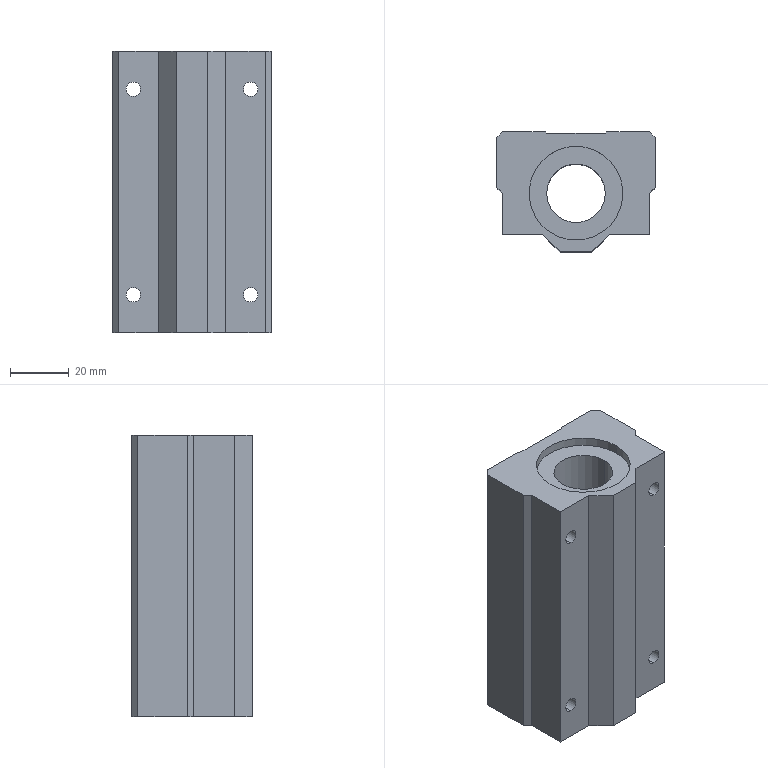Part | SolidWorks | features BaseBody 1 | 1 solid | 44 faces | box 54 x 41 x 96 mm | volume 148221 mm3 | plane 22 | cylinder 14 | cone 8 | commonest cylinder face diameters 4.917 x8 32 x4 20 x2
STEP:
#1=CARTESIAN_POINT('',(-10.,0.,-93.));
#2=VERTEX_POINT('',#1);
#3=CARTESIAN_POINT('',(10.,0.,-93.));
#4=VERTEX_POINT('',#3);
#5=CARTESIAN_POINT('',(0.,0.,-93.));
#6=DIRECTION('',(0.,0.,1.));
#7=DIRECTION('',(1.,0.,0.));
#8=AXIS2_PLACEMENT_3D('',#5,#6,#7);
#9=CIRCLE('',#8,10.);
#10=EDGE_CURVE('',#2,#4,#9,.T.);
#11=ORIENTED_EDGE('',*,*,#10,.F.);
#12=CARTESIAN_POINT('',(-10.,0.,-3.));
#13=VERTEX_POINT('',#12);
#14=CARTESIAN_POINT('',(-10.,0.,-96.));
#15=DIRECTION('',(0.,0.,1.));
#16=VECTOR('',#15,1000.);
#17=LINE('',#14,#16);
#18=EDGE_CURVE('',#2,#13,#17,.T.);
#19=ORIENTED_EDGE('',*,*,#18,.T.);
#20=CARTESIAN_POINT('',(10.,0.,-3.));
#21=VERTEX_POINT('',#20);
#22=CARTESIAN_POINT('',(0.,0.,-3.));
#23=DIRECTION('',(0.,0.,-1.));
#24=DIRECTION('',(1.,0.,0.));
#25=AXIS2_PLACEMENT_3D('',#22,#23,#24);
#26=CIRCLE('',#25,10.);
#27=EDGE_CURVE('',#21,#13,#26,.T.);
#28=ORIENTED_EDGE('',*,*,#27,.F.);
#29=CARTESIAN_POINT('',(10.,0.,-96.));
#30=DIRECTION('',(0.,0.,1.));
#31=VECTOR('',#30,1000.);
#32=LINE('',#29,#31);
#33=EDGE_CURVE('',#4,#21,#32,.T.);
#34=ORIENTED_EDGE('',*,*,#33,.F.);
#35=EDGE_LOOP('',(#11,#19,#28,#34));
#36=FACE_OUTER_BOUND('',#35,.T.);
#37=CARTESIAN_POINT('',(0.,0.,-96.));
#38=DIRECTION('',(0.,0.,1.));
#39=DIRECTION('',(1.,0.,0.));
#40=AXIS2_PLACEMENT_3D('',#37,#38,#39);
#41=CYLINDRICAL_SURFACE('',#40,10.);
#42=ADVANCED_FACE('',(#36),#41,.F.);
#43=CARTESIAN_POINT('',(-16.,0.,-3.));
#44=VERTEX_POINT('',#43);
#45=CARTESIAN_POINT('',(16.,0.,-3.));
#46=VERTEX_POINT('',#45);
#47=CARTESIAN_POINT('',(0.,0.,-3.));
#48=DIRECTION('',(0.,0.,1.));
#49=DIRECTION('',(1.,0.,0.));
#50=AXIS2_PLACEMENT_3D('',#47,#48,#49);
#51=CIRCLE('',#50,16.);
#52=EDGE_CURVE('',#44,#46,#51,.T.);
#53=ORIENTED_EDGE('',*,*,#52,.F.);
#54=CARTESIAN_POINT('',(-16.,0.,0.));
#55=VERTEX_POINT('',#54);
#56=CARTESIAN_POINT('',(-16.,0.,-96.));
#57=DIRECTION('',(0.,0.,1.));
#58=VECTOR('',#57,1000.);
#59=LINE('',#56,#58);
#60=EDGE_CURVE('',#44,#55,#59,.T.);
#61=ORIENTED_EDGE('',*,*,#60,.T.);
#62=CARTESIAN_POINT('',(16.,0.,0.));
#63=VERTEX_POINT('',#62);
#64=CARTESIAN_POINT('',(0.,0.,0.));
#65=DIRECTION('',(0.,0.,-1.));
#66=DIRECTION('',(1.,0.,0.));
#67=AXIS2_PLACEMENT_3D('',#64,#65,#66);
#68=CIRCLE('',#67,16.);
#69=EDGE_CURVE('',#63,#55,#68,.T.);
#70=ORIENTED_EDGE('',*,*,#69,.F.);
#71=CARTESIAN_POINT('',(16.,0.,-96.));
#72=DIRECTION('',(0.,0.,1.));
#73=VECTOR('',#72,1000.);
#74=LINE('',#71,#73);
#75=EDGE_CURVE('',#46,#63,#74,.T.);
#76=ORIENTED_EDGE('',*,*,#75,.F.);
#77=EDGE_LOOP('',(#53,#61,#70,#76));
#78=FACE_OUTER_BOUND('',#77,.T.);
#79=CARTESIAN_POINT('',(0.,0.,-96.));
#80=DIRECTION('',(0.,0.,1.));
#81=DIRECTION('',(1.,0.,0.));
#82=AXIS2_PLACEMENT_3D('',#79,#80,#81);
#83=CYLINDRICAL_SURFACE('',#82,16.);
#84=ADVANCED_FACE('',(#78),#83,.F.);
#85=CARTESIAN_POINT('',(-16.,0.,-96.));
#86=VERTEX_POINT('',#85);
#87=CARTESIAN_POINT('',(16.,0.,-96.));
#88=VERTEX_POINT('',#87);
#89=CARTESIAN_POINT('',(0.,0.,-96.));
#90=DIRECTION('',(0.,0.,1.));
#91=DIRECTION('',(1.,0.,0.));
#92=AXIS2_PLACEMENT_3D('',#89,#90,#91);
#93=CIRCLE('',#92,16.);
#94=EDGE_CURVE('',#86,#88,#93,.T.);
#95=ORIENTED_EDGE('',*,*,#94,.F.);
#96=CARTESIAN_POINT('',(-16.,0.,-93.));
#97=VERTEX_POINT('',#96);
#98=CARTESIAN_POINT('',(-16.,0.,-96.));
#99=DIRECTION('',(0.,0.,1.));
#100=VECTOR('',#99,1000.);
#101=LINE('',#98,#100);
#102=EDGE_CURVE('',#86,#97,#101,.T.);
#103=ORIENTED_EDGE('',*,*,#102,.T.);
#104=CARTESIAN_POINT('',(16.,0.,-93.));
#105=VERTEX_POINT('',#104);
#106=CARTESIAN_POINT('',(0.,0.,-93.));
#107=DIRECTION('',(0.,0.,-1.));
#108=DIRECTION('',(1.,0.,0.));
#109=AXIS2_PLACEMENT_3D('',#106,#107,#108);
#110=CIRCLE('',#109,16.);
#111=EDGE_CURVE('',#105,#97,#110,.T.);
#112=ORIENTED_EDGE('',*,*,#111,.F.);
#113=CARTESIAN_POINT('',(16.,0.,-96.));
#114=DIRECTION('',(0.,0.,1.));
#115=VECTOR('',#114,1000.);
#116=LINE('',#113,#115);
#117=EDGE_CURVE('',#88,#105,#116,.T.);
#118=ORIENTED_EDGE('',*,*,#117,.F.);
#119=EDGE_LOOP('',(#95,#103,#112,#118));
#120=FACE_OUTER_BOUND('',#119,.T.);
#121=CARTESIAN_POINT('',(0.,0.,-96.));
#122=DIRECTION('',(0.,0.,1.));
#123=DIRECTION('',(1.,0.,0.));
#124=AXIS2_PLACEMENT_3D('',#121,#122,#123);
#125=CYLINDRICAL_SURFACE('',#124,16.);
#126=ADVANCED_FACE('',(#120),#125,.F.);
#127=CARTESIAN_POINT('',(-20.,20.459,-85.459));
#128=VERTEX_POINT('',#127);
#129=CARTESIAN_POINT('',(-20.,20.459,-80.541));
#130=VERTEX_POINT('',#129);
#131=CARTESIAN_POINT('',(-20.,20.459,-83.));
#132=DIRECTION('',(0.,1.,0.));
#133=DIRECTION('',(0.,0.,1.));
#134=AXIS2_PLACEMENT_3D('',#131,#132,#133);
#135=CIRCLE('',#134,2.459);
#136=EDGE_CURVE('',#128,#130,#135,.T.);
#137=ORIENTED_EDGE('',*,*,#136,.F.);
#138=CARTESIAN_POINT('',(-20.,21.,-86.));
#139=VERTEX_POINT('',#138);
#140=CARTESIAN_POINT('',(-20.,21.,-86.));
#141=DIRECTION('',(0.,0.7071,-0.7071));
#142=VECTOR('',#141,1000.);
#143=LINE('',#140,#142);
#144=EDGE_CURVE('',#128,#139,#143,.T.);
#145=ORIENTED_EDGE('',*,*,#144,.T.);
#146=CARTESIAN_POINT('',(-20.,21.,-80.));
#147=VERTEX_POINT('',#146);
#148=CARTESIAN_POINT('',(-20.,21.,-83.));
#149=DIRECTION('',(0.,-1.,0.));
#150=DIRECTION('',(0.,0.,1.));
#151=AXIS2_PLACEMENT_3D('',#148,#149,#150);
#152=CIRCLE('',#151,3.);
#153=EDGE_CURVE('',#147,#139,#152,.T.);
#154=ORIENTED_EDGE('',*,*,#153,.F.);
#155=CARTESIAN_POINT('',(-20.,21.,-80.));
#156=DIRECTION('',(0.,0.7071,0.7071));
#157=VECTOR('',#156,1000.);
#158=LINE('',#155,#157);
#159=EDGE_CURVE('',#130,#147,#158,.T.);
#160=ORIENTED_EDGE('',*,*,#159,.F.);
#161=EDGE_LOOP('',(#137,#145,#154,#160));
#162=FACE_OUTER_BOUND('',#161,.T.);
#163=CARTESIAN_POINT('',(-20.,21.,-83.));
#164=DIRECTION('',(0.,1.,0.));
#165=DIRECTION('',(0.,0.,1.));
#166=AXIS2_PLACEMENT_3D('',#163,#164,#165);
#167=CONICAL_SURFACE('',#166,3.,0.7854);
#168=ADVANCED_FACE('',(#162),#167,.F.);
#169=CARTESIAN_POINT('',(-20.,20.459,-15.459));
#170=VERTEX_POINT('',#169);
#171=CARTESIAN_POINT('',(-20.,20.459,-10.541));
#172=VERTEX_POINT('',#171);
#173=CARTESIAN_POINT('',(-20.,20.459,-13.));
#174=DIRECTION('',(0.,1.,0.));
#175=DIRECTION('',(0.,0.,1.));
#176=AXIS2_PLACEMENT_3D('',#173,#174,#175);
#177=CIRCLE('',#176,2.459);
#178=EDGE_CURVE('',#170,#172,#177,.T.);
#179=ORIENTED_EDGE('',*,*,#178,.F.);
#180=CARTESIAN_POINT('',(-20.,21.,-16.));
#181=VERTEX_POINT('',#180);
#182=CARTESIAN_POINT('',(-20.,21.,-16.));
#183=DIRECTION('',(0.,0.7071,-0.7071));
#184=VECTOR('',#183,1000.);
#185=LINE('',#182,#184);
#186=EDGE_CURVE('',#170,#181,#185,.T.);
#187=ORIENTED_EDGE('',*,*,#186,.T.);
#188=CARTESIAN_POINT('',(-20.,21.,-10.));
#189=VERTEX_POINT('',#188);
#190=CARTESIAN_POINT('',(-20.,21.,-13.));
#191=DIRECTION('',(0.,-1.,0.));
#192=DIRECTION('',(0.,0.,1.));
#193=AXIS2_PLACEMENT_3D('',#190,#191,#192);
#194=CIRCLE('',#193,3.);
#195=EDGE_CURVE('',#189,#181,#194,.T.);
#196=ORIENTED_EDGE('',*,*,#195,.F.);
#197=CARTESIAN_POINT('',(-20.,21.,-10.));
#198=DIRECTION('',(0.,0.7071,0.7071));
#199=VECTOR('',#198,1000.);
#200=LINE('',#197,#199);
#201=EDGE_CURVE('',#172,#189,#200,.T.);
#202=ORIENTED_EDGE('',*,*,#201,.F.);
#203=EDGE_LOOP('',(#179,#187,#196,#202));
#204=FACE_OUTER_BOUND('',#203,.T.);
#205=CARTESIAN_POINT('',(-20.,21.,-13.));
#206=DIRECTION('',(0.,1.,0.));
#207=DIRECTION('',(0.,0.,1.));
#208=AXIS2_PLACEMENT_3D('',#205,#206,#207);
#209=CONICAL_SURFACE('',#208,3.,0.7854);
#210=ADVANCED_FACE('',(#204),#209,.F.);
#211=CARTESIAN_POINT('',(20.,20.458,-85.459));
#212=VERTEX_POINT('',#211);
#213=CARTESIAN_POINT('',(20.,20.458,-80.541));
#214=VERTEX_POINT('',#213);
#215=CARTESIAN_POINT('',(20.,20.458,-83.));
#216=DIRECTION('',(0.,1.,0.));
#217=DIRECTION('',(0.,0.,1.));
#218=AXIS2_PLACEMENT_3D('',#215,#216,#217);
#219=CIRCLE('',#218,2.459);
#220=EDGE_CURVE('',#212,#214,#219,.T.);
#221=ORIENTED_EDGE('',*,*,#220,.F.);
#222=CARTESIAN_POINT('',(20.,21.,-86.));
#223=VERTEX_POINT('',#222);
#224=CARTESIAN_POINT('',(20.,21.,-86.));
#225=DIRECTION('',(0.,0.7071,-0.7071));
#226=VECTOR('',#225,1000.);
#227=LINE('',#224,#226);
#228=EDGE_CURVE('',#212,#223,#227,.T.);
#229=ORIENTED_EDGE('',*,*,#228,.T.);
#230=CARTESIAN_POINT('',(20.,21.,-80.));
#231=VERTEX_POINT('',#230);
#232=CARTESIAN_POINT('',(20.,21.,-83.));
#233=DIRECTION('',(0.,-1.,0.));
#234=DIRECTION('',(0.,0.,1.));
#235=AXIS2_PLACEMENT_3D('',#232,#233,#234);
#236=CIRCLE('',#235,3.);
#237=EDGE_CURVE('',#231,#223,#236,.T.);
#238=ORIENTED_EDGE('',*,*,#237,.F.);
#239=CARTESIAN_POINT('',(20.,21.,-80.));
#240=DIRECTION('',(0.,0.7071,0.7071));
#241=VECTOR('',#240,1000.);
#242=LINE('',#239,#241);
#243=EDGE_CURVE('',#214,#231,#242,.T.);
#244=ORIENTED_EDGE('',*,*,#243,.F.);
#245=EDGE_LOOP('',(#221,#229,#238,#244));
#246=FACE_OUTER_BOUND('',#245,.T.);
#247=CARTESIAN_POINT('',(20.,21.,-83.));
#248=DIRECTION('',(0.,1.,0.));
#249=DIRECTION('',(0.,0.,1.));
#250=AXIS2_PLACEMENT_3D('',#247,#248,#249);
#251=CONICAL_SURFACE('',#250,3.,0.7854);
#252=ADVANCED_FACE('',(#246),#251,.F.);
#253=CARTESIAN_POINT('',(20.,20.458,-15.459));
#254=VERTEX_POINT('',#253);
#255=CARTESIAN_POINT('',(20.,20.458,-10.541));
#256=VERTEX_POINT('',#255);
#257=CARTESIAN_POINT('',(20.,20.458,-13.));
#258=DIRECTION('',(0.,1.,0.));
#259=DIRECTION('',(0.,0.,1.));
#260=AXIS2_PLACEMENT_3D('',#257,#258,#259);
#261=CIRCLE('',#260,2.459);
#262=EDGE_CURVE('',#254,#256,#261,.T.);
#263=ORIENTED_EDGE('',*,*,#262,.F.);
#264=CARTESIAN_POINT('',(20.,21.,-16.));
#265=VERTEX_POINT('',#264);
#266=CARTESIAN_POINT('',(20.,21.,-16.));
#267=DIRECTION('',(0.,0.7071,-0.7071));
#268=VECTOR('',#267,1000.);
#269=LINE('',#266,#268);
#270=EDGE_CURVE('',#254,#265,#269,.T.);
#271=ORIENTED_EDGE('',*,*,#270,.T.);
#272=CARTESIAN_POINT('',(20.,21.,-10.));
#273=VERTEX_POINT('',#272);
#274=CARTESIAN_POINT('',(20.,21.,-13.));
#275=DIRECTION('',(0.,-1.,0.));
#276=DIRECTION('',(0.,0.,1.));
#277=AXIS2_PLACEMENT_3D('',#274,#275,#276);
#278=CIRCLE('',#277,3.);
#279=EDGE_CURVE('',#273,#265,#278,.T.);
#280=ORIENTED_EDGE('',*,*,#279,.F.);
#281=CARTESIAN_POINT('',(20.,21.,-10.));
#282=DIRECTION('',(0.,0.7071,0.7071));
#283=VECTOR('',#282,1000.);
#284=LINE('',#281,#283);
#285=EDGE_CURVE('',#256,#273,#284,.T.);
#286=ORIENTED_EDGE('',*,*,#285,.F.);
#287=EDGE_LOOP('',(#263,#271,#280,#286));
#288=FACE_OUTER_BOUND('',#287,.T.);
#289=CARTESIAN_POINT('',(20.,21.,-13.));
#290=DIRECTION('',(0.,1.,0.));
#291=DIRECTION('',(0.,0.,1.));
#292=AXIS2_PLACEMENT_3D('',#289,#290,#291);
#293=CONICAL_SURFACE('',#292,3.,0.7854);
#294=ADVANCED_FACE('',(#288),#293,.F.);
#295=CARTESIAN_POINT('',(20.,-14.,-85.459));
#296=VERTEX_POINT('',#295);
#297=CARTESIAN_POINT('',(20.,-14.,-80.541));
#298=VERTEX_POINT('',#297);
#299=CARTESIAN_POINT('',(20.,-14.,-83.));
#300=DIRECTION('',(0.,1.,0.));
#301=DIRECTION('',(0.,0.,1.));
#302=AXIS2_PLACEMENT_3D('',#299,#300,#301);
#303=CIRCLE('',#302,2.459);
#304=EDGE_CURVE('',#296,#298,#303,.T.);
#305=ORIENTED_EDGE('',*,*,#304,.F.);
#306=CARTESIAN_POINT('',(20.,-14.,-85.459));
#307=DIRECTION('',(0.,1.,0.));
#308=VECTOR('',#307,1000.);
#309=LINE('',#306,#308);
#310=EDGE_CURVE('',#296,#212,#309,.T.);
#311=ORIENTED_EDGE('',*,*,#310,.T.);
#312=ORIENTED_EDGE('',*,*,#220,.T.);
#313=CARTESIAN_POINT('',(20.,-14.,-80.541));
#314=DIRECTION('',(0.,1.,0.));
#315=VECTOR('',#314,1000.);
#316=LINE('',#313,#315);
#317=EDGE_CURVE('',#298,#214,#316,.T.);
#318=ORIENTED_EDGE('',*,*,#317,.F.);
#319=EDGE_LOOP('',(#305,#311,#312,#318));
#320=FACE_OUTER_BOUND('',#319,.T.);
#321=CARTESIAN_POINT('',(20.,-14.,-83.));
#322=DIRECTION('',(0.,1.,0.));
#323=DIRECTION('',(0.,0.,1.));
#324=AXIS2_PLACEMENT_3D('',#321,#322,#323);
#325=CYLINDRICAL_SURFACE('',#324,2.459);
#326=ADVANCED_FACE('',(#320),#325,.F.);
#327=CARTESIAN_POINT('',(20.,-14.,-15.459));
#328=VERTEX_POINT('',#327);
#329=CARTESIAN_POINT('',(20.,-14.,-10.542));
#330=VERTEX_POINT('',#329);
#331=CARTESIAN_POINT('',(20.,-14.,-13.));
#332=DIRECTION('',(0.,1.,0.));
#333=DIRECTION('',(0.,0.,1.));
#334=AXIS2_PLACEMENT_3D('',#331,#332,#333);
#335=CIRCLE('',#334,2.458);
#336=EDGE_CURVE('',#328,#330,#335,.T.);
#337=ORIENTED_EDGE('',*,*,#336,.F.);
#338=CARTESIAN_POINT('',(20.,-14.,-15.459));
#339=DIRECTION('',(0.,1.,0.));
#340=VECTOR('',#339,1000.);
#341=LINE('',#338,#340);
#342=EDGE_CURVE('',#328,#254,#341,.T.);
#343=ORIENTED_EDGE('',*,*,#342,.T.);
#344=ORIENTED_EDGE('',*,*,#262,.T.);
#345=CARTESIAN_POINT('',(20.,-14.,-10.542));
#346=DIRECTION('',(0.,1.,0.));
#347=VECTOR('',#346,1000.);
#348=LINE('',#345,#347);
#349=EDGE_CURVE('',#330,#256,#348,.T.);
#350=ORIENTED_EDGE('',*,*,#349,.F.);
#351=EDGE_LOOP('',(#337,#343,#344,#350));
#352=FACE_OUTER_BOUND('',#351,.T.);
#353=CARTESIAN_POINT('',(20.,-14.,-13.));
#354=DIRECTION('',(0.,1.,0.));
#355=DIRECTION('',(0.,0.,1.));
#356=AXIS2_PLACEMENT_3D('',#353,#354,#355);
#357=CYLINDRICAL_SURFACE('',#356,2.458);
#358=ADVANCED_FACE('',(#352),#357,.F.);
#359=ORIENTED_EDGE('',*,*,#136,.T.);
#360=CARTESIAN_POINT('',(-20.,-14.,-80.541));
#361=VERTEX_POINT('',#360);
#362=CARTESIAN_POINT('',(-20.,21.,-80.541));
#363=DIRECTION('',(0.,-1.,0.));
#364=VECTOR('',#363,1000.);
#365=LINE('',#362,#364);
#366=EDGE_CURVE('',#130,#361,#365,.T.);
#367=ORIENTED_EDGE('',*,*,#366,.T.);
#368=CARTESIAN_POINT('',(-20.,-14.,-85.459));
#369=VERTEX_POINT('',#368);
#370=CARTESIAN_POINT('',(-20.,-14.,-83.));
#371=DIRECTION('',(0.,1.,0.));
#372=DIRECTION('',(0.,0.,-1.));
#373=AXIS2_PLACEMENT_3D('',#370,#371,#372);
#374=CIRCLE('',#373,2.459);
#375=EDGE_CURVE('',#369,#361,#374,.T.);
#376=ORIENTED_EDGE('',*,*,#375,.F.);
#377=CARTESIAN_POINT('',(-20.,21.,-85.459));
#378=DIRECTION('',(0.,-1.,0.));
#379=VECTOR('',#378,1000.);
#380=LINE('',#377,#379);
#381=EDGE_CURVE('',#128,#369,#380,.T.);
#382=ORIENTED_EDGE('',*,*,#381,.F.);
#383=EDGE_LOOP('',(#359,#367,#376,#382));
#384=FACE_OUTER_BOUND('',#383,.T.);
#385=CARTESIAN_POINT('',(-20.,21.,-83.));
#386=DIRECTION('',(0.,-1.,0.));
#387=DIRECTION('',(0.,0.,-1.));
#388=AXIS2_PLACEMENT_3D('',#385,#386,#387);
#389=CYLINDRICAL_SURFACE('',#388,2.459);
#390=ADVANCED_FACE('',(#384),#389,.F.);
#391=ORIENTED_EDGE('',*,*,#178,.T.);
#392=CARTESIAN_POINT('',(-20.,-14.,-10.542));
#393=VERTEX_POINT('',#392);
#394=CARTESIAN_POINT('',(-20.,21.,-10.542));
#395=DIRECTION('',(0.,-1.,0.));
#396=VECTOR('',#395,1000.);
#397=LINE('',#394,#396);
#398=EDGE_CURVE('',#172,#393,#397,.T.);
#399=ORIENTED_EDGE('',*,*,#398,.T.);
#400=CARTESIAN_POINT('',(-20.,-14.,-15.459));
#401=VERTEX_POINT('',#400);
#402=CARTESIAN_POINT('',(-20.,-14.,-13.));
#403=DIRECTION('',(0.,1.,0.));
#404=DIRECTION('',(0.,0.,-1.));
#405=AXIS2_PLACEMENT_3D('',#402,#403,#404);
#406=CIRCLE('',#405,2.458);
#407=EDGE_CURVE('',#401,#393,#406,.T.);
#408=ORIENTED_EDGE('',*,*,#407,.F.);
#409=CARTESIAN_POINT('',(-20.,21.,-15.459));
#410=DIRECTION('',(0.,-1.,0.));
#411=VECTOR('',#410,1000.);
#412=LINE('',#409,#411);
#413=EDGE_CURVE('',#170,#401,#412,.T.);
#414=ORIENTED_EDGE('',*,*,#413,.F.);
#415=EDGE_LOOP('',(#391,#399,#408,#414));
#416=FACE_OUTER_BOUND('',#415,.T.);
#417=CARTESIAN_POINT('',(-20.,21.,-13.));
#418=DIRECTION('',(0.,-1.,0.));
#419=DIRECTION('',(0.,0.,-1.));
#420=AXIS2_PLACEMENT_3D('',#417,#418,#419);
#421=CYLINDRICAL_SURFACE('',#420,2.458);
#422=ADVANCED_FACE('',(#416),#421,.F.);
#423=ORIENTED_EDGE('',*,*,#18,.F.);
#424=CARTESIAN_POINT('',(0.,0.,-93.));
#425=DIRECTION('',(0.,0.,1.));
#426=DIRECTION('',(1.,0.,0.));
#427=AXIS2_PLACEMENT_3D('',#424,#425,#426);
#428=CIRCLE('',#427,10.);
#429=EDGE_CURVE('',#4,#2,#428,.T.);
#430=ORIENTED_EDGE('',*,*,#429,.F.);
#431=ORIENTED_EDGE('',*,*,#33,.T.);
#432=CARTESIAN_POINT('',(0.,0.,-3.));
#433=DIRECTION('',(0.,0.,-1.));
#434=DIRECTION('',(1.,0.,0.));
#435=AXIS2_PLACEMENT_3D('',#432,#433,#434);
#436=CIRCLE('',#435,10.);
#437=EDGE_CURVE('',#13,#21,#436,.T.);
#438=ORIENTED_EDGE('',*,*,#437,.F.);
#439=EDGE_LOOP('',(#423,#430,#431,#438));
#440=FACE_OUTER_BOUND('',#439,.T.);
#441=CARTESIAN_POINT('',(0.,0.,-96.));
#442=DIRECTION('',(0.,0.,1.));
#443=DIRECTION('',(1.,0.,0.));
#444=AXIS2_PLACEMENT_3D('',#441,#442,#443);
#445=CYLINDRICAL_SURFACE('',#444,10.);
#446=ADVANCED_FACE('',(#440),#445,.F.);
#447=CARTESIAN_POINT('',(0.,0.,-3.));
#448=DIRECTION('',(0.,0.,1.));
#449=DIRECTION('',(1.,0.,0.));
#450=AXIS2_PLACEMENT_3D('',#447,#448,#449);
#451=CIRCLE('',#450,16.);
#452=EDGE_CURVE('',#46,#44,#451,.T.);
#453=ORIENTED_EDGE('',*,*,#452,.T.);
#454=ORIENTED_EDGE('',*,*,#52,.T.);
#455=EDGE_LOOP('',(#453,#454));
#456=FACE_OUTER_BOUND('',#455,.T.);
#457=ORIENTED_EDGE('',*,*,#27,.T.);
#458=ORIENTED_EDGE('',*,*,#437,.T.);
#459=EDGE_LOOP('',(#457,#458));
#460=FACE_BOUND('',#459,.T.);
#461=CARTESIAN_POINT('',(0.,16.,-3.));
#462=DIRECTION('',(0.,0.,1.));
#463=DIRECTION('',(1.,0.,0.));
#464=AXIS2_PLACEMENT_3D('',#461,#462,#463);
#465=PLANE('',#464);
#466=ADVANCED_FACE('',(#456,#460),#465,.T.);
#467=ORIENTED_EDGE('',*,*,#429,.T.);
#468=ORIENTED_EDGE('',*,*,#10,.T.);
#469=EDGE_LOOP('',(#467,#468));
#470=FACE_BOUND('',#469,.T.);
#471=ORIENTED_EDGE('',*,*,#111,.T.);
#472=CARTESIAN_POINT('',(0.,0.,-93.));
#473=DIRECTION('',(0.,0.,-1.));
#474=DIRECTION('',(1.,0.,0.));
#475=AXIS2_PLACEMENT_3D('',#472,#473,#474);
#476=CIRCLE('',#475,16.);
#477=EDGE_CURVE('',#97,#105,#476,.T.);
#478=ORIENTED_EDGE('',*,*,#477,.T.);
#479=EDGE_LOOP('',(#471,#478));
#480=FACE_OUTER_BOUND('',#479,.T.);
#481=CARTESIAN_POINT('',(0.,10.,-93.));
#482=DIRECTION('',(0.,0.,-1.));
#483=DIRECTION('',(-1.,0.,0.));
#484=AXIS2_PLACEMENT_3D('',#481,#482,#483);
#485=PLANE('',#484);
#486=ADVANCED_FACE('',(#470,#480),#485,.T.);
#487=ORIENTED_EDGE('',*,*,#60,.F.);
#488=ORIENTED_EDGE('',*,*,#452,.F.);
#489=ORIENTED_EDGE('',*,*,#75,.T.);
#490=CARTESIAN_POINT('',(0.,0.,0.));
#491=DIRECTION('',(0.,0.,-1.));
#492=DIRECTION('',(1.,0.,0.));
#493=AXIS2_PLACEMENT_3D('',#490,#491,#492);
#494=CIRCLE('',#493,16.);
#495=EDGE_CURVE('',#55,#63,#494,.T.);
#496=ORIENTED_EDGE('',*,*,#495,.F.);
#497=EDGE_LOOP('',(#487,#488,#489,#496));
#498=FACE_OUTER_BOUND('',#497,.T.);
#499=CARTESIAN_POINT('',(0.,0.,-96.));
#500=DIRECTION('',(0.,0.,1.));
#501=DIRECTION('',(1.,0.,0.));
#502=AXIS2_PLACEMENT_3D('',#499,#500,#501);
#503=CYLINDRICAL_SURFACE('',#502,16.);
#504=ADVANCED_FACE('',(#498),#503,.F.);
#505=ORIENTED_EDGE('',*,*,#102,.F.);
#506=CARTESIAN_POINT('',(0.,0.,-96.));
#507=DIRECTION('',(0.,0.,1.));
#508=DIRECTION('',(1.,0.,0.));
#509=AXIS2_PLACEMENT_3D('',#506,#507,#508);
#510=CIRCLE('',#509,16.);
#511=EDGE_CURVE('',#88,#86,#510,.T.);
#512=ORIENTED_EDGE('',*,*,#511,.F.);
#513=ORIENTED_EDGE('',*,*,#117,.T.);
#514=ORIENTED_EDGE('',*,*,#477,.F.);
#515=EDGE_LOOP('',(#505,#512,#513,#514));
#516=FACE_OUTER_BOUND('',#515,.T.);
#517=CARTESIAN_POINT('',(0.,0.,-96.));
#518=DIRECTION('',(0.,0.,1.));
#519=DIRECTION('',(1.,0.,0.));
#520=AXIS2_PLACEMENT_3D('',#517,#518,#519);
#521=CYLINDRICAL_SURFACE('',#520,16.);
#522=ADVANCED_FACE('',(#516),#521,.F.);
#523=ORIENTED_EDGE('',*,*,#69,.T.);
#524=ORIENTED_EDGE('',*,*,#495,.T.);
#525=EDGE_LOOP('',(#523,#524));
#526=FACE_BOUND('',#525,.T.);
#527=CARTESIAN_POINT('',(-10.5,21.,0.));
#528=VERTEX_POINT('',#527);
#529=CARTESIAN_POINT('',(-25.,21.,0.));
#530=VERTEX_POINT('',#529);
#531=CARTESIAN_POINT('',(0.,21.,0.));
#532=DIRECTION('',(-1.,0.,0.));
#533=VECTOR('',#532,1000.);
#534=LINE('',#531,#533);
#535=EDGE_CURVE('',#528,#530,#534,.T.);
#536=ORIENTED_EDGE('',*,*,#535,.T.);
#537=CARTESIAN_POINT('',(-27.,19.,0.));
#538=VERTEX_POINT('',#537);
#539=CARTESIAN_POINT('',(-25.,21.,0.));
#540=DIRECTION('',(-0.7071,-0.7071,0.));
#541=VECTOR('',#540,1000.);
#542=LINE('',#539,#541);
#543=EDGE_CURVE('',#530,#538,#542,.T.);
#544=ORIENTED_EDGE('',*,*,#543,.T.);
#545=CARTESIAN_POINT('',(-27.,2.,0.));
#546=VERTEX_POINT('',#545);
#547=CARTESIAN_POINT('',(-27.,0.,0.));
#548=DIRECTION('',(0.,-1.,0.));
#549=VECTOR('',#548,1000.);
#550=LINE('',#547,#549);
#551=EDGE_CURVE('',#538,#546,#550,.T.);
#552=ORIENTED_EDGE('',*,*,#551,.T.);
#553=CARTESIAN_POINT('',(-25.,0.,0.));
#554=VERTEX_POINT('',#553);
#555=CARTESIAN_POINT('',(-27.,2.,0.));
#556=DIRECTION('',(0.7071,-0.7071,0.));
#557=VECTOR('',#556,1000.);
#558=LINE('',#555,#557);
#559=EDGE_CURVE('',#546,#554,#558,.T.);
#560=ORIENTED_EDGE('',*,*,#559,.T.);
#561=CARTESIAN_POINT('',(-25.,-14.,0.));
#562=VERTEX_POINT('',#561);
#563=CARTESIAN_POINT('',(-25.,0.,0.));
#564=DIRECTION('',(0.,-1.,0.));
#565=VECTOR('',#564,1000.);
#566=LINE('',#563,#565);
#567=EDGE_CURVE('',#554,#562,#566,.T.);
#568=ORIENTED_EDGE('',*,*,#567,.T.);
#569=CARTESIAN_POINT('',(-11.4,-14.,0.));
#570=VERTEX_POINT('',#569);
#571=CARTESIAN_POINT('',(0.,-14.,0.));
#572=DIRECTION('',(1.,0.,0.));
#573=VECTOR('',#572,1000.);
#574=LINE('',#571,#573);
#575=EDGE_CURVE('',#562,#570,#574,.T.);
#576=ORIENTED_EDGE('',*,*,#575,.T.);
#577=CARTESIAN_POINT('',(-5.4,-20.,0.));
#578=VERTEX_POINT('',#577);
#579=CARTESIAN_POINT('',(-11.4,-14.,0.));
#580=DIRECTION('',(0.7071,-0.7071,0.));
#581=VECTOR('',#580,1000.);
#582=LINE('',#579,#581);
#583=EDGE_CURVE('',#570,#578,#582,.T.);
#584=ORIENTED_EDGE('',*,*,#583,.T.);
#585=CARTESIAN_POINT('',(5.4,-20.,0.));
#586=VERTEX_POINT('',#585);
#587=CARTESIAN_POINT('',(0.,-20.,0.));
#588=DIRECTION('',(1.,0.,0.));
#589=VECTOR('',#588,1000.);
#590=LINE('',#587,#589);
#591=EDGE_CURVE('',#578,#586,#590,.T.);
#592=ORIENTED_EDGE('',*,*,#591,.T.);
#593=CARTESIAN_POINT('',(11.4,-14.,0.));
#594=VERTEX_POINT('',#593);
#595=CARTESIAN_POINT('',(5.4,-20.,0.));
#596=DIRECTION('',(0.7071,0.7071,0.));
#597=VECTOR('',#596,1000.);
#598=LINE('',#595,#597);
#599=EDGE_CURVE('',#586,#594,#598,.T.);
#600=ORIENTED_EDGE('',*,*,#599,.T.);
#601=CARTESIAN_POINT('',(25.,-14.,0.));
#602=VERTEX_POINT('',#601);
#603=CARTESIAN_POINT('',(0.,-14.,0.));
#604=DIRECTION('',(1.,0.,0.));
#605=VECTOR('',#604,1000.);
#606=LINE('',#603,#605);
#607=EDGE_CURVE('',#594,#602,#606,.T.);
#608=ORIENTED_EDGE('',*,*,#607,.T.);
#609=CARTESIAN_POINT('',(25.,0.,0.));
#610=VERTEX_POINT('',#609);
#611=CARTESIAN_POINT('',(25.,0.,0.));
#612=DIRECTION('',(0.,1.,0.));
#613=VECTOR('',#612,1000.);
#614=LINE('',#611,#613);
#615=EDGE_CURVE('',#602,#610,#614,.T.);
#616=ORIENTED_EDGE('',*,*,#615,.T.);
#617=CARTESIAN_POINT('',(27.,2.,0.));
#618=VERTEX_POINT('',#617);
#619=CARTESIAN_POINT('',(25.,0.,0.));
#620=DIRECTION('',(0.7071,0.7071,0.));
#621=VECTOR('',#620,1000.);
#622=LINE('',#619,#621);
#623=EDGE_CURVE('',#610,#618,#622,.T.);
#624=ORIENTED_EDGE('',*,*,#623,.T.);
#625=CARTESIAN_POINT('',(27.,19.,0.));
#626=VERTEX_POINT('',#625);
#627=CARTESIAN_POINT('',(27.,0.,0.));
#628=DIRECTION('',(0.,1.,0.));
#629=VECTOR('',#628,1000.);
#630=LINE('',#627,#629);
#631=EDGE_CURVE('',#618,#626,#630,.T.);
#632=ORIENTED_EDGE('',*,*,#631,.T.);
#633=CARTESIAN_POINT('',(25.,21.,0.));
#634=VERTEX_POINT('',#633);
#635=CARTESIAN_POINT('',(27.,19.,0.));
#636=DIRECTION('',(-0.7071,0.7071,0.));
#637=VECTOR('',#636,1000.);
#638=LINE('',#635,#637);
#639=EDGE_CURVE('',#626,#634,#638,.T.);
#640=ORIENTED_EDGE('',*,*,#639,.T.);
#641=CARTESIAN_POINT('',(10.5,21.,0.));
#642=VERTEX_POINT('',#641);
#643=CARTESIAN_POINT('',(0.,21.,0.));
#644=DIRECTION('',(-1.,0.,0.));
#645=VECTOR('',#644,1000.);
#646=LINE('',#643,#645);
#647=EDGE_CURVE('',#634,#642,#646,.T.);
#648=ORIENTED_EDGE('',*,*,#647,.T.);
#649=CARTESIAN_POINT('',(10.,20.5,0.));
#650=VERTEX_POINT('',#649);
#651=CARTESIAN_POINT('',(10.5,21.,0.));
#652=DIRECTION('',(0.7071,0.7071,0.));
#653=VECTOR('',#652,1000.);
#654=LINE('',#651,#653);
#655=EDGE_CURVE('',#650,#642,#654,.T.);
#656=ORIENTED_EDGE('',*,*,#655,.F.);
#657=CARTESIAN_POINT('',(-10.,20.5,0.));
#658=VERTEX_POINT('',#657);
#659=CARTESIAN_POINT('',(0.,20.5,0.));
#660=DIRECTION('',(-1.,0.,0.));
#661=VECTOR('',#660,1000.);
#662=LINE('',#659,#661);
#663=EDGE_CURVE('',#650,#658,#662,.T.);
#664=ORIENTED_EDGE('',*,*,#663,.T.);
#665=CARTESIAN_POINT('',(-10.,20.5,0.));
#666=DIRECTION('',(0.7071,-0.7071,0.));
#667=VECTOR('',#666,1000.);
#668=LINE('',#665,#667);
#669=EDGE_CURVE('',#528,#658,#668,.T.);
#670=ORIENTED_EDGE('',*,*,#669,.F.);
#671=EDGE_LOOP('',(#536,#544,#552,#560,#568,#576,#584,#592,#600,#608,#616,#624,#632,#640,#648,#656,#664,#670));
#672=FACE_OUTER_BOUND('',#671,.T.);
#673=CARTESIAN_POINT('',(0.,0.,0.));
#674=DIRECTION('',(0.,0.,1.));
#675=DIRECTION('',(1.,0.,0.));
#676=AXIS2_PLACEMENT_3D('',#673,#674,#675);
#677=PLANE('',#676);
#678=ADVANCED_FACE('',(#526,#672),#677,.T.);
#679=ORIENTED_EDGE('',*,*,#511,.T.);
#680=ORIENTED_EDGE('',*,*,#94,.T.);
#681=EDGE_LOOP('',(#679,#680));
#682=FACE_BOUND('',#681,.T.);
#683=CARTESIAN_POINT('',(-25.,21.,-96.));
#684=VERTEX_POINT('',#683);
#685=CARTESIAN_POINT('',(-27.,19.,-96.));
#686=VERTEX_POINT('',#685);
#687=CARTESIAN_POINT('',(-25.,21.,-96.));
#688=DIRECTION('',(-0.7071,-0.7071,0.));
#689=VECTOR('',#688,1000.);
#690=LINE('',#687,#689);
#691=EDGE_CURVE('',#684,#686,#690,.T.);
#692=ORIENTED_EDGE('',*,*,#691,.F.);
#693=CARTESIAN_POINT('',(-10.5,21.,-96.));
#694=VERTEX_POINT('',#693);
#695=CARTESIAN_POINT('',(0.,21.,-96.));
#696=DIRECTION('',(-1.,0.,0.));
#697=VECTOR('',#696,1000.);
#698=LINE('',#695,#697);
#699=EDGE_CURVE('',#694,#684,#698,.T.);
#700=ORIENTED_EDGE('',*,*,#699,.F.);
#701=CARTESIAN_POINT('',(-10.,20.5,-96.));
#702=VERTEX_POINT('',#701);
#703=CARTESIAN_POINT('',(-10.,20.5,-96.));
#704=DIRECTION('',(-0.7071,0.7071,0.));
#705=VECTOR('',#704,1000.);
#706=LINE('',#703,#705);
#707=EDGE_CURVE('',#702,#694,#706,.T.);
#708=ORIENTED_EDGE('',*,*,#707,.F.);
#709=CARTESIAN_POINT('',(10.,20.5,-96.));
#710=VERTEX_POINT('',#709);
#711=CARTESIAN_POINT('',(0.,20.5,-96.));
#712=DIRECTION('',(-1.,0.,0.));
#713=VECTOR('',#712,1000.);
#714=LINE('',#711,#713);
#715=EDGE_CURVE('',#710,#702,#714,.T.);
#716=ORIENTED_EDGE('',*,*,#715,.F.);
#717=CARTESIAN_POINT('',(10.5,21.,-96.));
#718=VERTEX_POINT('',#717);
#719=CARTESIAN_POINT('',(10.5,21.,-96.));
#720=DIRECTION('',(-0.7071,-0.7071,0.));
#721=VECTOR('',#720,1000.);
#722=LINE('',#719,#721);
#723=EDGE_CURVE('',#718,#710,#722,.T.);
#724=ORIENTED_EDGE('',*,*,#723,.F.);
#725=CARTESIAN_POINT('',(25.,21.,-96.));
#726=VERTEX_POINT('',#725);
#727=CARTESIAN_POINT('',(0.,21.,-96.));
#728=DIRECTION('',(-1.,0.,0.));
#729=VECTOR('',#728,1000.);
#730=LINE('',#727,#729);
#731=EDGE_CURVE('',#726,#718,#730,.T.);
#732=ORIENTED_EDGE('',*,*,#731,.F.);
#733=CARTESIAN_POINT('',(27.,19.,-96.));
#734=VERTEX_POINT('',#733);
#735=CARTESIAN_POINT('',(27.,19.,-96.));
#736=DIRECTION('',(-0.7071,0.7071,0.));
#737=VECTOR('',#736,1000.);
#738=LINE('',#735,#737);
#739=EDGE_CURVE('',#734,#726,#738,.T.);
#740=ORIENTED_EDGE('',*,*,#739,.F.);
#741=CARTESIAN_POINT('',(27.,2.,-96.));
#742=VERTEX_POINT('',#741);
#743=CARTESIAN_POINT('',(27.,0.,-96.));
#744=DIRECTION('',(0.,1.,0.));
#745=VECTOR('',#744,1000.);
#746=LINE('',#743,#745);
#747=EDGE_CURVE('',#742,#734,#746,.T.);
#748=ORIENTED_EDGE('',*,*,#747,.F.);
#749=CARTESIAN_POINT('',(25.,0.,-96.));
#750=VERTEX_POINT('',#749);
#751=CARTESIAN_POINT('',(25.,0.,-96.));
#752=DIRECTION('',(0.7071,0.7071,0.));
#753=VECTOR('',#752,1000.);
#754=LINE('',#751,#753);
#755=EDGE_CURVE('',#750,#742,#754,.T.);
#756=ORIENTED_EDGE('',*,*,#755,.F.);
#757=CARTESIAN_POINT('',(25.,-14.,-96.));
#758=VERTEX_POINT('',#757);
#759=CARTESIAN_POINT('',(25.,0.,-96.));
#760=DIRECTION('',(0.,1.,0.));
#761=VECTOR('',#760,1000.);
#762=LINE('',#759,#761);
#763=EDGE_CURVE('',#758,#750,#762,.T.);
#764=ORIENTED_EDGE('',*,*,#763,.F.);
#765=CARTESIAN_POINT('',(11.4,-14.,-96.));
#766=VERTEX_POINT('',#765);
#767=CARTESIAN_POINT('',(0.,-14.,-96.));
#768=DIRECTION('',(1.,0.,0.));
#769=VECTOR('',#768,1000.);
#770=LINE('',#767,#769);
#771=EDGE_CURVE('',#766,#758,#770,.T.);
#772=ORIENTED_EDGE('',*,*,#771,.F.);
#773=CARTESIAN_POINT('',(5.4,-20.,-96.));
#774=VERTEX_POINT('',#773);
#775=CARTESIAN_POINT('',(5.4,-20.,-96.));
#776=DIRECTION('',(0.7071,0.7071,0.));
#777=VECTOR('',#776,1000.);
#778=LINE('',#775,#777);
#779=EDGE_CURVE('',#774,#766,#778,.T.);
#780=ORIENTED_EDGE('',*,*,#779,.F.);
#781=CARTESIAN_POINT('',(-5.4,-20.,-96.));
#782=VERTEX_POINT('',#781);
#783=CARTESIAN_POINT('',(0.,-20.,-96.));
#784=DIRECTION('',(1.,0.,0.));
#785=VECTOR('',#784,1000.);
#786=LINE('',#783,#785);
#787=EDGE_CURVE('',#782,#774,#786,.T.);
#788=ORIENTED_EDGE('',*,*,#787,.F.);
#789=CARTESIAN_POINT('',(-11.4,-14.,-96.));
#790=VERTEX_POINT('',#789);
#791=CARTESIAN_POINT('',(-11.4,-14.,-96.));
#792=DIRECTION('',(0.7071,-0.7071,0.));
#793=VECTOR('',#792,1000.);
#794=LINE('',#791,#793);
#795=EDGE_CURVE('',#790,#782,#794,.T.);
#796=ORIENTED_EDGE('',*,*,#795,.F.);
#797=CARTESIAN_POINT('',(-25.,-14.,-96.));
#798=VERTEX_POINT('',#797);
#799=CARTESIAN_POINT('',(0.,-14.,-96.));
#800=DIRECTION('',(1.,0.,0.));
#801=VECTOR('',#800,1000.);
#802=LINE('',#799,#801);
#803=EDGE_CURVE('',#798,#790,#802,.T.);
#804=ORIENTED_EDGE('',*,*,#803,.F.);
#805=CARTESIAN_POINT('',(-25.,0.,-96.));
#806=VERTEX_POINT('',#805);
#807=CARTESIAN_POINT('',(-25.,0.,-96.));
#808=DIRECTION('',(0.,-1.,0.));
#809=VECTOR('',#808,1000.);
#810=LINE('',#807,#809);
#811=EDGE_CURVE('',#806,#798,#810,.T.);
#812=ORIENTED_EDGE('',*,*,#811,.F.);
#813=CARTESIAN_POINT('',(-27.,2.,-96.));
#814=VERTEX_POINT('',#813);
#815=CARTESIAN_POINT('',(-27.,2.,-96.));
#816=DIRECTION('',(0.7071,-0.7071,0.));
#817=VECTOR('',#816,1000.);
#818=LINE('',#815,#817);
#819=EDGE_CURVE('',#814,#806,#818,.T.);
#820=ORIENTED_EDGE('',*,*,#819,.F.);
#821=CARTESIAN_POINT('',(-27.,0.,-96.));
#822=DIRECTION('',(0.,-1.,0.));
#823=VECTOR('',#822,1000.);
#824=LINE('',#821,#823);
#825=EDGE_CURVE('',#686,#814,#824,.T.);
#826=ORIENTED_EDGE('',*,*,#825,.F.);
#827=EDGE_LOOP('',(#692,#700,#708,#716,#724,#732,#740,#748,#756,#764,#772,#780,#788,#796,#804,#812,#820,#826));
#828=FACE_OUTER_BOUND('',#827,.T.);
#829=CARTESIAN_POINT('',(0.,0.,-96.));
#830=DIRECTION('',(0.,0.,1.));
#831=DIRECTION('',(1.,0.,0.));
#832=AXIS2_PLACEMENT_3D('',#829,#830,#831);
#833=PLANE('',#832);
#834=ADVANCED_FACE('',(#682,#828),#833,.F.);
#835=ORIENTED_EDGE('',*,*,#691,.T.);
#836=CARTESIAN_POINT('',(-27.,19.,-96.));
#837=DIRECTION('',(0.,0.,1.));
#838=VECTOR('',#837,1000.);
#839=LINE('',#836,#838);
#840=EDGE_CURVE('',#686,#538,#839,.T.);
#841=ORIENTED_EDGE('',*,*,#840,.T.);
#842=ORIENTED_EDGE('',*,*,#543,.F.);
#843=CARTESIAN_POINT('',(-25.,21.,-96.));
#844=DIRECTION('',(0.,0.,-1.));
#845=VECTOR('',#844,1000.);
#846=LINE('',#843,#845);
#847=EDGE_CURVE('',#530,#684,#846,.T.);
#848=ORIENTED_EDGE('',*,*,#847,.T.);
#849=EDGE_LOOP('',(#835,#841,#842,#848));
#850=FACE_OUTER_BOUND('',#849,.T.);
#851=CARTESIAN_POINT('',(-25.,21.,-96.));
#852=DIRECTION('',(-0.7071,0.7071,0.));
#853=DIRECTION('',(-0.7071,-0.7071,0.));
#854=AXIS2_PLACEMENT_3D('',#851,#852,#853);
#855=PLANE('',#854);
#856=ADVANCED_FACE('',(#850),#855,.T.);
#857=ORIENTED_EDGE('',*,*,#153,.T.);
#858=CARTESIAN_POINT('',(-20.,21.,-83.));
#859=DIRECTION('',(0.,-1.,0.));
#860=DIRECTION('',(0.,0.,1.));
#861=AXIS2_PLACEMENT_3D('',#858,#859,#860);
#862=CIRCLE('',#861,3.);
#863=EDGE_CURVE('',#139,#147,#862,.T.);
#864=ORIENTED_EDGE('',*,*,#863,.T.);
#865=EDGE_LOOP('',(#857,#864));
#866=FACE_BOUND('',#865,.T.);
#867=ORIENTED_EDGE('',*,*,#699,.T.);
#868=ORIENTED_EDGE('',*,*,#847,.F.);
#869=ORIENTED_EDGE('',*,*,#535,.F.);
#870=CARTESIAN_POINT('',(-10.5,21.,-96.));
#871=DIRECTION('',(0.,0.,-1.));
#872=VECTOR('',#871,1000.);
#873=LINE('',#870,#872);
#874=EDGE_CURVE('',#528,#694,#873,.T.);
#875=ORIENTED_EDGE('',*,*,#874,.T.);
#876=EDGE_LOOP('',(#867,#868,#869,#875));
#877=FACE_OUTER_BOUND('',#876,.T.);
#878=ORIENTED_EDGE('',*,*,#195,.T.);
#879=CARTESIAN_POINT('',(-20.,21.,-13.));
#880=DIRECTION('',(0.,-1.,0.));
#881=DIRECTION('',(0.,0.,1.));
#882=AXIS2_PLACEMENT_3D('',#879,#880,#881);
#883=CIRCLE('',#882,3.);
#884=EDGE_CURVE('',#181,#189,#883,.T.);
#885=ORIENTED_EDGE('',*,*,#884,.T.);
#886=EDGE_LOOP('',(#878,#885));
#887=FACE_BOUND('',#886,.T.);
#888=CARTESIAN_POINT('',(-10.5,21.,-96.));
#889=DIRECTION('',(0.,1.,0.));
#890=DIRECTION('',(0.,0.,1.));
#891=AXIS2_PLACEMENT_3D('',#888,#889,#890);
#892=PLANE('',#891);
#893=ADVANCED_FACE('',(#866,#877,#887),#892,.T.);
#894=ORIENTED_EDGE('',*,*,#715,.T.);
#895=CARTESIAN_POINT('',(-10.,20.5,-96.));
#896=DIRECTION('',(0.,0.,1.));
#897=VECTOR('',#896,1000.);
#898=LINE('',#895,#897);
#899=EDGE_CURVE('',#702,#658,#898,.T.);
#900=ORIENTED_EDGE('',*,*,#899,.T.);
#901=ORIENTED_EDGE('',*,*,#663,.F.);
#902=CARTESIAN_POINT('',(10.,20.5,-96.));
#903=DIRECTION('',(0.,0.,-1.));
#904=VECTOR('',#903,1000.);
#905=LINE('',#902,#904);
#906=EDGE_CURVE('',#650,#710,#905,.T.);
#907=ORIENTED_EDGE('',*,*,#906,.T.);
#908=EDGE_LOOP('',(#894,#900,#901,#907));
#909=FACE_OUTER_BOUND('',#908,.T.);
#910=CARTESIAN_POINT('',(10.,20.5,-96.));
#911=DIRECTION('',(0.,1.,0.));
#912=DIRECTION('',(0.,0.,1.));
#913=AXIS2_PLACEMENT_3D('',#910,#911,#912);
#914=PLANE('',#913);
#915=ADVANCED_FACE('',(#909),#914,.T.);
#916=ORIENTED_EDGE('',*,*,#237,.T.);
#917=CARTESIAN_POINT('',(20.,21.,-83.));
#918=DIRECTION('',(0.,-1.,0.));
#919=DIRECTION('',(0.,0.,1.));
#920=AXIS2_PLACEMENT_3D('',#917,#918,#919);
#921=CIRCLE('',#920,3.);
#922=EDGE_CURVE('',#223,#231,#921,.T.);
#923=ORIENTED_EDGE('',*,*,#922,.T.);
#924=EDGE_LOOP('',(#916,#923));
#925=FACE_BOUND('',#924,.T.);
#926=ORIENTED_EDGE('',*,*,#731,.T.);
#927=CARTESIAN_POINT('',(10.5,21.,-96.));
#928=DIRECTION('',(0.,0.,1.));
#929=VECTOR('',#928,1000.);
#930=LINE('',#927,#929);
#931=EDGE_CURVE('',#718,#642,#930,.T.);
#932=ORIENTED_EDGE('',*,*,#931,.T.);
#933=ORIENTED_EDGE('',*,*,#647,.F.);
#934=CARTESIAN_POINT('',(25.,21.,-96.));
#935=DIRECTION('',(0.,0.,-1.));
#936=VECTOR('',#935,1000.);
#937=LINE('',#934,#936);
#938=EDGE_CURVE('',#634,#726,#937,.T.);
#939=ORIENTED_EDGE('',*,*,#938,.T.);
#940=EDGE_LOOP('',(#926,#932,#933,#939));
#941=FACE_OUTER_BOUND('',#940,.T.);
#942=ORIENTED_EDGE('',*,*,#279,.T.);
#943=CARTESIAN_POINT('',(20.,21.,-13.));
#944=DIRECTION('',(0.,-1.,0.));
#945=DIRECTION('',(0.,0.,1.));
#946=AXIS2_PLACEMENT_3D('',#943,#944,#945);
#947=CIRCLE('',#946,3.);
#948=EDGE_CURVE('',#265,#273,#947,.T.);
#949=ORIENTED_EDGE('',*,*,#948,.T.);
#950=EDGE_LOOP('',(#942,#949));
#951=FACE_BOUND('',#950,.T.);
#952=CARTESIAN_POINT('',(25.,21.,-96.));
#953=DIRECTION('',(0.,1.,0.));
#954=DIRECTION('',(0.,0.,1.));
#955=AXIS2_PLACEMENT_3D('',#952,#953,#954);
#956=PLANE('',#955);
#957=ADVANCED_FACE('',(#925,#941,#951),#956,.T.);
#958=ORIENTED_EDGE('',*,*,#739,.T.);
#959=ORIENTED_EDGE('',*,*,#938,.F.);
#960=ORIENTED_EDGE('',*,*,#639,.F.);
#961=CARTESIAN_POINT('',(27.,19.,-96.));
#962=DIRECTION('',(0.,0.,-1.));
#963=VECTOR('',#962,1000.);
#964=LINE('',#961,#963);
#965=EDGE_CURVE('',#626,#734,#964,.T.);
#966=ORIENTED_EDGE('',*,*,#965,.T.);
#967=EDGE_LOOP('',(#958,#959,#960,#966));
#968=FACE_OUTER_BOUND('',#967,.T.);
#969=CARTESIAN_POINT('',(27.,19.,-96.));
#970=DIRECTION('',(0.7071,0.7071,0.));
#971=DIRECTION('',(-0.7071,0.7071,0.));
#972=AXIS2_PLACEMENT_3D('',#969,#970,#971);
#973=PLANE('',#972);
#974=ADVANCED_FACE('',(#968),#973,.T.);
#975=ORIENTED_EDGE('',*,*,#747,.T.);
#976=ORIENTED_EDGE('',*,*,#965,.F.);
#977=ORIENTED_EDGE('',*,*,#631,.F.);
#978=CARTESIAN_POINT('',(27.,2.,-96.));
#979=DIRECTION('',(0.,0.,-1.));
#980=VECTOR('',#979,1000.);
#981=LINE('',#978,#980);
#982=EDGE_CURVE('',#618,#742,#981,.T.);
#983=ORIENTED_EDGE('',*,*,#982,.T.);
#984=EDGE_LOOP('',(#975,#976,#977,#983));
#985=FACE_OUTER_BOUND('',#984,.T.);
#986=CARTESIAN_POINT('',(27.,2.,-96.));
#987=DIRECTION('',(1.,0.,0.));
#988=DIRECTION('',(0.,0.,-1.));
#989=AXIS2_PLACEMENT_3D('',#986,#987,#988);
#990=PLANE('',#989);
#991=ADVANCED_FACE('',(#985),#990,.T.);
#992=ORIENTED_EDGE('',*,*,#755,.T.);
#993=ORIENTED_EDGE('',*,*,#982,.F.);
#994=ORIENTED_EDGE('',*,*,#623,.F.);
#995=CARTESIAN_POINT('',(25.,0.,-96.));
#996=DIRECTION('',(0.,0.,-1.));
#997=VECTOR('',#996,1000.);
#998=LINE('',#995,#997);
#999=EDGE_CURVE('',#610,#750,#998,.T.);
#1000=ORIENTED_EDGE('',*,*,#999,.T.);
#1001=EDGE_LOOP('',(#992,#993,#994,#1000));
#1002=FACE_OUTER_BOUND('',#1001,.T.);
#1003=CARTESIAN_POINT('',(25.,0.,-96.));
#1004=DIRECTION('',(0.7071,-0.7071,0.));
#1005=DIRECTION('',(0.7071,0.7071,0.));
#1006=AXIS2_PLACEMENT_3D('',#1003,#1004,#1005);
#1007=PLANE('',#1006);
#1008=ADVANCED_FACE('',(#1002),#1007,.T.);
#1009=ORIENTED_EDGE('',*,*,#763,.T.);
#1010=ORIENTED_EDGE('',*,*,#999,.F.);
#1011=ORIENTED_EDGE('',*,*,#615,.F.);
#1012=CARTESIAN_POINT('',(25.,-14.,-96.));
#1013=DIRECTION('',(0.,0.,-1.));
#1014=VECTOR('',#1013,1000.);
#1015=LINE('',#1012,#1014);
#1016=EDGE_CURVE('',#602,#758,#1015,.T.);
#1017=ORIENTED_EDGE('',*,*,#1016,.T.);
#1018=EDGE_LOOP('',(#1009,#1010,#1011,#1017));
#1019=FACE_OUTER_BOUND('',#1018,.T.);
#1020=CARTESIAN_POINT('',(25.,-14.,-96.));
#1021=DIRECTION('',(1.,0.,0.));
#1022=DIRECTION('',(0.,0.,-1.));
#1023=AXIS2_PLACEMENT_3D('',#1020,#1021,#1022);
#1024=PLANE('',#1023);
#1025=ADVANCED_FACE('',(#1019),#1024,.T.);
#1026=CARTESIAN_POINT('',(20.,-14.,-83.));
#1027=DIRECTION('',(0.,1.,0.));
#1028=DIRECTION('',(0.,0.,1.));
#1029=AXIS2_PLACEMENT_3D('',#1026,#1027,#1028);
#1030=CIRCLE('',#1029,2.459);
#1031=EDGE_CURVE('',#298,#296,#1030,.T.);
#1032=ORIENTED_EDGE('',*,*,#1031,.T.);
#1033=ORIENTED_EDGE('',*,*,#304,.T.);
#1034=EDGE_LOOP('',(#1032,#1033));
#1035=FACE_BOUND('',#1034,.T.);
#1036=ORIENTED_EDGE('',*,*,#771,.T.);
#1037=ORIENTED_EDGE('',*,*,#1016,.F.);
#1038=ORIENTED_EDGE('',*,*,#607,.F.);
#1039=CARTESIAN_POINT('',(11.4,-14.,-96.));
#1040=DIRECTION('',(0.,0.,-1.));
#1041=VECTOR('',#1040,1000.);
#1042=LINE('',#1039,#1041);
#1043=EDGE_CURVE('',#594,#766,#1042,.T.);
#1044=ORIENTED_EDGE('',*,*,#1043,.T.);
#1045=EDGE_LOOP('',(#1036,#1037,#1038,#1044));
#1046=FACE_OUTER_BOUND('',#1045,.T.);
#1047=CARTESIAN_POINT('',(20.,-14.,-13.));
#1048=DIRECTION('',(0.,1.,0.));
#1049=DIRECTION('',(0.,0.,1.));
#1050=AXIS2_PLACEMENT_3D('',#1047,#1048,#1049);
#1051=CIRCLE('',#1050,2.458);
#1052=EDGE_CURVE('',#330,#328,#1051,.T.);
#1053=ORIENTED_EDGE('',*,*,#1052,.T.);
#1054=ORIENTED_EDGE('',*,*,#336,.T.);
#1055=EDGE_LOOP('',(#1053,#1054));
#1056=FACE_BOUND('',#1055,.T.);
#1057=CARTESIAN_POINT('',(11.4,-14.,-96.));
#1058=DIRECTION('',(0.,-1.,0.));
#1059=DIRECTION('',(0.,0.,-1.));
#1060=AXIS2_PLACEMENT_3D('',#1057,#1058,#1059);
#1061=PLANE('',#1060);
#1062=ADVANCED_FACE('',(#1035,#1046,#1056),#1061,.T.);
#1063=ORIENTED_EDGE('',*,*,#779,.T.);
#1064=ORIENTED_EDGE('',*,*,#1043,.F.);
#1065=ORIENTED_EDGE('',*,*,#599,.F.);
#1066=CARTESIAN_POINT('',(5.4,-20.,-96.));
#1067=DIRECTION('',(0.,0.,-1.));
#1068=VECTOR('',#1067,1000.);
#1069=LINE('',#1066,#1068);
#1070=EDGE_CURVE('',#586,#774,#1069,.T.);
#1071=ORIENTED_EDGE('',*,*,#1070,.T.);
#1072=EDGE_LOOP('',(#1063,#1064,#1065,#1071));
#1073=FACE_OUTER_BOUND('',#1072,.T.);
#1074=CARTESIAN_POINT('',(5.4,-20.,-96.));
#1075=DIRECTION('',(0.7071,-0.7071,0.));
#1076=DIRECTION('',(0.7071,0.7071,0.));
#1077=AXIS2_PLACEMENT_3D('',#1074,#1075,#1076);
#1078=PLANE('',#1077);
#1079=ADVANCED_FACE('',(#1073),#1078,.T.);
#1080=ORIENTED_EDGE('',*,*,#787,.T.);
#1081=ORIENTED_EDGE('',*,*,#1070,.F.);
#1082=ORIENTED_EDGE('',*,*,#591,.F.);
#1083=CARTESIAN_POINT('',(-5.4,-20.,-96.));
#1084=DIRECTION('',(0.,0.,-1.));
#1085=VECTOR('',#1084,1000.);
#1086=LINE('',#1083,#1085);
#1087=EDGE_CURVE('',#578,#782,#1086,.T.);
#1088=ORIENTED_EDGE('',*,*,#1087,.T.);
#1089=EDGE_LOOP('',(#1080,#1081,#1082,#1088));
#1090=FACE_OUTER_BOUND('',#1089,.T.);
#1091=CARTESIAN_POINT('',(-5.4,-20.,-96.));
#1092=DIRECTION('',(0.,-1.,0.));
#1093=DIRECTION('',(0.,0.,-1.));
#1094=AXIS2_PLACEMENT_3D('',#1091,#1092,#1093);
#1095=PLANE('',#1094);
#1096=ADVANCED_FACE('',(#1090),#1095,.T.);
#1097=ORIENTED_EDGE('',*,*,#795,.T.);
#1098=ORIENTED_EDGE('',*,*,#1087,.F.);
#1099=ORIENTED_EDGE('',*,*,#583,.F.);
#1100=CARTESIAN_POINT('',(-11.4,-14.,-96.));
#1101=DIRECTION('',(0.,0.,-1.));
#1102=VECTOR('',#1101,1000.);
#1103=LINE('',#1100,#1102);
#1104=EDGE_CURVE('',#570,#790,#1103,.T.);
#1105=ORIENTED_EDGE('',*,*,#1104,.T.);
#1106=EDGE_LOOP('',(#1097,#1098,#1099,#1105));
#1107=FACE_OUTER_BOUND('',#1106,.T.);
#1108=CARTESIAN_POINT('',(-11.4,-14.,-96.));
#1109=DIRECTION('',(-0.7071,-0.7071,0.));
#1110=DIRECTION('',(0.7071,-0.7071,0.));
#1111=AXIS2_PLACEMENT_3D('',#1108,#1109,#1110);
#1112=PLANE('',#1111);
#1113=ADVANCED_FACE('',(#1107),#1112,.T.);
#1114=ORIENTED_EDGE('',*,*,#375,.T.);
#1115=CARTESIAN_POINT('',(-20.,-14.,-83.));
#1116=DIRECTION('',(0.,1.,0.));
#1117=DIRECTION('',(0.,0.,-1.));
#1118=AXIS2_PLACEMENT_3D('',#1115,#1116,#1117);
#1119=CIRCLE('',#1118,2.459);
#1120=EDGE_CURVE('',#361,#369,#1119,.T.);
#1121=ORIENTED_EDGE('',*,*,#1120,.T.);
#1122=EDGE_LOOP('',(#1114,#1121));
#1123=FACE_BOUND('',#1122,.T.);
#1124=ORIENTED_EDGE('',*,*,#803,.T.);
#1125=ORIENTED_EDGE('',*,*,#1104,.F.);
#1126=ORIENTED_EDGE('',*,*,#575,.F.);
#1127=CARTESIAN_POINT('',(-25.,-14.,-96.));
#1128=DIRECTION('',(0.,0.,-1.));
#1129=VECTOR('',#1128,1000.);
#1130=LINE('',#1127,#1129);
#1131=EDGE_CURVE('',#562,#798,#1130,.T.);
#1132=ORIENTED_EDGE('',*,*,#1131,.T.);
#1133=EDGE_LOOP('',(#1124,#1125,#1126,#1132));
#1134=FACE_OUTER_BOUND('',#1133,.T.);
#1135=ORIENTED_EDGE('',*,*,#407,.T.);
#1136=CARTESIAN_POINT('',(-20.,-14.,-13.));
#1137=DIRECTION('',(0.,1.,0.));
#1138=DIRECTION('',(0.,0.,-1.));
#1139=AXIS2_PLACEMENT_3D('',#1136,#1137,#1138);
#1140=CIRCLE('',#1139,2.458);
#1141=EDGE_CURVE('',#393,#401,#1140,.T.);
#1142=ORIENTED_EDGE('',*,*,#1141,.T.);
#1143=EDGE_LOOP('',(#1135,#1142));
#1144=FACE_BOUND('',#1143,.T.);
#1145=CARTESIAN_POINT('',(-25.,-14.,-96.));
#1146=DIRECTION('',(0.,-1.,0.));
#1147=DIRECTION('',(0.,0.,-1.));
#1148=AXIS2_PLACEMENT_3D('',#1145,#1146,#1147);
#1149=PLANE('',#1148);
#1150=ADVANCED_FACE('',(#1123,#1134,#1144),#1149,.T.);
#1151=ORIENTED_EDGE('',*,*,#811,.T.);
#1152=ORIENTED_EDGE('',*,*,#1131,.F.);
#1153=ORIENTED_EDGE('',*,*,#567,.F.);
#1154=CARTESIAN_POINT('',(-25.,0.,-96.));
#1155=DIRECTION('',(0.,0.,-1.));
#1156=VECTOR('',#1155,1000.);
#1157=LINE('',#1154,#1156);
#1158=EDGE_CURVE('',#554,#806,#1157,.T.);
#1159=ORIENTED_EDGE('',*,*,#1158,.T.);
#1160=EDGE_LOOP('',(#1151,#1152,#1153,#1159));
#1161=FACE_OUTER_BOUND('',#1160,.T.);
#1162=CARTESIAN_POINT('',(-25.,0.,-96.));
#1163=DIRECTION('',(-1.,0.,0.));
#1164=DIRECTION('',(0.,0.,1.));
#1165=AXIS2_PLACEMENT_3D('',#1162,#1163,#1164);
#1166=PLANE('',#1165);
#1167=ADVANCED_FACE('',(#1161),#1166,.T.);
#1168=ORIENTED_EDGE('',*,*,#819,.T.);
#1169=ORIENTED_EDGE('',*,*,#1158,.F.);
#1170=ORIENTED_EDGE('',*,*,#559,.F.);
#1171=CARTESIAN_POINT('',(-27.,2.,-96.));
#1172=DIRECTION('',(0.,0.,-1.));
#1173=VECTOR('',#1172,1000.);
#1174=LINE('',#1171,#1173);
#1175=EDGE_CURVE('',#546,#814,#1174,.T.);
#1176=ORIENTED_EDGE('',*,*,#1175,.T.);
#1177=EDGE_LOOP('',(#1168,#1169,#1170,#1176));
#1178=FACE_OUTER_BOUND('',#1177,.T.);
#1179=CARTESIAN_POINT('',(-27.,2.,-96.));
#1180=DIRECTION('',(-0.7071,-0.7071,0.));
#1181=DIRECTION('',(0.7071,-0.7071,0.));
#1182=AXIS2_PLACEMENT_3D('',#1179,#1180,#1181);
#1183=PLANE('',#1182);
#1184=ADVANCED_FACE('',(#1178),#1183,.T.);
#1185=ORIENTED_EDGE('',*,*,#825,.T.);
#1186=ORIENTED_EDGE('',*,*,#1175,.F.);
#1187=ORIENTED_EDGE('',*,*,#551,.F.);
#1188=ORIENTED_EDGE('',*,*,#840,.F.);
#1189=EDGE_LOOP('',(#1185,#1186,#1187,#1188));
#1190=FACE_OUTER_BOUND('',#1189,.T.);
#1191=CARTESIAN_POINT('',(-27.,19.,-96.));
#1192=DIRECTION('',(-1.,0.,0.));
#1193=DIRECTION('',(0.,0.,1.));
#1194=AXIS2_PLACEMENT_3D('',#1191,#1192,#1193);
#1195=PLANE('',#1194);
#1196=ADVANCED_FACE('',(#1190),#1195,.T.);
#1197=ORIENTED_EDGE('',*,*,#144,.F.);
#1198=CARTESIAN_POINT('',(-20.,20.459,-83.));
#1199=DIRECTION('',(0.,1.,0.));
#1200=DIRECTION('',(0.,0.,1.));
#1201=AXIS2_PLACEMENT_3D('',#1198,#1199,#1200);
#1202=CIRCLE('',#1201,2.459);
#1203=EDGE_CURVE('',#130,#128,#1202,.T.);
#1204=ORIENTED_EDGE('',*,*,#1203,.F.);
#1205=ORIENTED_EDGE('',*,*,#159,.T.);
#1206=ORIENTED_EDGE('',*,*,#863,.F.);
#1207=EDGE_LOOP('',(#1197,#1204,#1205,#1206));
#1208=FACE_OUTER_BOUND('',#1207,.T.);
#1209=CARTESIAN_POINT('',(-20.,21.,-83.));
#1210=DIRECTION('',(0.,1.,0.));
#1211=DIRECTION('',(0.,0.,1.));
#1212=AXIS2_PLACEMENT_3D('',#1209,#1210,#1211);
#1213=CONICAL_SURFACE('',#1212,3.,0.7854);
#1214=ADVANCED_FACE('',(#1208),#1213,.F.);
#1215=ORIENTED_EDGE('',*,*,#707,.T.);
#1216=ORIENTED_EDGE('',*,*,#874,.F.);
#1217=ORIENTED_EDGE('',*,*,#669,.T.);
#1218=ORIENTED_EDGE('',*,*,#899,.F.);
#1219=EDGE_LOOP('',(#1215,#1216,#1217,#1218));
#1220=FACE_OUTER_BOUND('',#1219,.T.);
#1221=CARTESIAN_POINT('',(-10.,20.5,-96.));
#1222=DIRECTION('',(0.7071,0.7071,0.));
#1223=DIRECTION('',(-0.7071,0.7071,0.));
#1224=AXIS2_PLACEMENT_3D('',#1221,#1222,#1223);
#1225=PLANE('',#1224);
#1226=ADVANCED_FACE('',(#1220),#1225,.T.);
#1227=ORIENTED_EDGE('',*,*,#186,.F.);
#1228=CARTESIAN_POINT('',(-20.,20.459,-13.));
#1229=DIRECTION('',(0.,1.,0.));
#1230=DIRECTION('',(0.,0.,1.));
#1231=AXIS2_PLACEMENT_3D('',#1228,#1229,#1230);
#1232=CIRCLE('',#1231,2.459);
#1233=EDGE_CURVE('',#172,#170,#1232,.T.);
#1234=ORIENTED_EDGE('',*,*,#1233,.F.);
#1235=ORIENTED_EDGE('',*,*,#201,.T.);
#1236=ORIENTED_EDGE('',*,*,#884,.F.);
#1237=EDGE_LOOP('',(#1227,#1234,#1235,#1236));
#1238=FACE_OUTER_BOUND('',#1237,.T.);
#1239=CARTESIAN_POINT('',(-20.,21.,-13.));
#1240=DIRECTION('',(0.,1.,0.));
#1241=DIRECTION('',(0.,0.,1.));
#1242=AXIS2_PLACEMENT_3D('',#1239,#1240,#1241);
#1243=CONICAL_SURFACE('',#1242,3.,0.7854);
#1244=ADVANCED_FACE('',(#1238),#1243,.F.);
#1245=ORIENTED_EDGE('',*,*,#723,.T.);
#1246=ORIENTED_EDGE('',*,*,#906,.F.);
#1247=ORIENTED_EDGE('',*,*,#655,.T.);
#1248=ORIENTED_EDGE('',*,*,#931,.F.);
#1249=EDGE_LOOP('',(#1245,#1246,#1247,#1248));
#1250=FACE_OUTER_BOUND('',#1249,.T.);
#1251=CARTESIAN_POINT('',(10.5,21.,-96.));
#1252=DIRECTION('',(-0.7071,0.7071,0.));
#1253=DIRECTION('',(-0.7071,-0.7071,0.));
#1254=AXIS2_PLACEMENT_3D('',#1251,#1252,#1253);
#1255=PLANE('',#1254);
#1256=ADVANCED_FACE('',(#1250),#1255,.T.);
#1257=ORIENTED_EDGE('',*,*,#228,.F.);
#1258=CARTESIAN_POINT('',(20.,20.458,-83.));
#1259=DIRECTION('',(0.,1.,0.));
#1260=DIRECTION('',(0.,0.,1.));
#1261=AXIS2_PLACEMENT_3D('',#1258,#1259,#1260);
#1262=CIRCLE('',#1261,2.459);
#1263=EDGE_CURVE('',#214,#212,#1262,.T.);
#1264=ORIENTED_EDGE('',*,*,#1263,.F.);
#1265=ORIENTED_EDGE('',*,*,#243,.T.);
#1266=ORIENTED_EDGE('',*,*,#922,.F.);
#1267=EDGE_LOOP('',(#1257,#1264,#1265,#1266));
#1268=FACE_OUTER_BOUND('',#1267,.T.);
#1269=CARTESIAN_POINT('',(20.,21.,-83.));
#1270=DIRECTION('',(0.,1.,0.));
#1271=DIRECTION('',(0.,0.,1.));
#1272=AXIS2_PLACEMENT_3D('',#1269,#1270,#1271);
#1273=CONICAL_SURFACE('',#1272,3.,0.7854);
#1274=ADVANCED_FACE('',(#1268),#1273,.F.);
#1275=ORIENTED_EDGE('',*,*,#270,.F.);
#1276=CARTESIAN_POINT('',(20.,20.458,-13.));
#1277=DIRECTION('',(0.,1.,0.));
#1278=DIRECTION('',(0.,0.,1.));
#1279=AXIS2_PLACEMENT_3D('',#1276,#1277,#1278);
#1280=CIRCLE('',#1279,2.459);
#1281=EDGE_CURVE('',#256,#254,#1280,.T.);
#1282=ORIENTED_EDGE('',*,*,#1281,.F.);
#1283=ORIENTED_EDGE('',*,*,#285,.T.);
#1284=ORIENTED_EDGE('',*,*,#948,.F.);
#1285=EDGE_LOOP('',(#1275,#1282,#1283,#1284));
#1286=FACE_OUTER_BOUND('',#1285,.T.);
#1287=CARTESIAN_POINT('',(20.,21.,-13.));
#1288=DIRECTION('',(0.,1.,0.));
#1289=DIRECTION('',(0.,0.,1.));
#1290=AXIS2_PLACEMENT_3D('',#1287,#1288,#1289);
#1291=CONICAL_SURFACE('',#1290,3.,0.7854);
#1292=ADVANCED_FACE('',(#1286),#1291,.F.);
#1293=ORIENTED_EDGE('',*,*,#310,.F.);
#1294=ORIENTED_EDGE('',*,*,#1031,.F.);
#1295=ORIENTED_EDGE('',*,*,#317,.T.);
#1296=ORIENTED_EDGE('',*,*,#1263,.T.);
#1297=EDGE_LOOP('',(#1293,#1294,#1295,#1296));
#1298=FACE_OUTER_BOUND('',#1297,.T.);
#1299=CARTESIAN_POINT('',(20.,-14.,-83.));
#1300=DIRECTION('',(0.,1.,0.));
#1301=DIRECTION('',(0.,0.,1.));
#1302=AXIS2_PLACEMENT_3D('',#1299,#1300,#1301);
#1303=CYLINDRICAL_SURFACE('',#1302,2.459);
#1304=ADVANCED_FACE('',(#1298),#1303,.F.);
#1305=ORIENTED_EDGE('',*,*,#342,.F.);
#1306=ORIENTED_EDGE('',*,*,#1052,.F.);
#1307=ORIENTED_EDGE('',*,*,#349,.T.);
#1308=ORIENTED_EDGE('',*,*,#1281,.T.);
#1309=EDGE_LOOP('',(#1305,#1306,#1307,#1308));
#1310=FACE_OUTER_BOUND('',#1309,.T.);
#1311=CARTESIAN_POINT('',(20.,-14.,-13.));
#1312=DIRECTION('',(0.,1.,0.));
#1313=DIRECTION('',(0.,0.,1.));
#1314=AXIS2_PLACEMENT_3D('',#1311,#1312,#1313);
#1315=CYLINDRICAL_SURFACE('',#1314,2.458);
#1316=ADVANCED_FACE('',(#1310),#1315,.F.);
#1317=ORIENTED_EDGE('',*,*,#366,.F.);
#1318=ORIENTED_EDGE('',*,*,#1203,.T.);
#1319=ORIENTED_EDGE('',*,*,#381,.T.);
#1320=ORIENTED_EDGE('',*,*,#1120,.F.);
#1321=EDGE_LOOP('',(#1317,#1318,#1319,#1320));
#1322=FACE_OUTER_BOUND('',#1321,.T.);
#1323=CARTESIAN_POINT('',(-20.,21.,-83.));
#1324=DIRECTION('',(0.,-1.,0.));
#1325=DIRECTION('',(0.,0.,-1.));
#1326=AXIS2_PLACEMENT_3D('',#1323,#1324,#1325);
#1327=CYLINDRICAL_SURFACE('',#1326,2.459);
#1328=ADVANCED_FACE('',(#1322),#1327,.F.);
#1329=ORIENTED_EDGE('',*,*,#398,.F.);
#1330=ORIENTED_EDGE('',*,*,#1233,.T.);
#1331=ORIENTED_EDGE('',*,*,#413,.T.);
#1332=ORIENTED_EDGE('',*,*,#1141,.F.);
#1333=EDGE_LOOP('',(#1329,#1330,#1331,#1332));
#1334=FACE_OUTER_BOUND('',#1333,.T.);
#1335=CARTESIAN_POINT('',(-20.,21.,-13.));
#1336=DIRECTION('',(0.,-1.,0.));
#1337=DIRECTION('',(0.,0.,-1.));
#1338=AXIS2_PLACEMENT_3D('',#1335,#1336,#1337);
#1339=CYLINDRICAL_SURFACE('',#1338,2.458);
#1340=ADVANCED_FACE('',(#1334),#1339,.F.);
#1341=CLOSED_SHELL('',(#42,#84,#126,#168,#210,#252,#294,#326,#358,#390,#422,#446,#466,#486,#504,#522,#678,#834,#856,#893,#915,#957,#974,#991,#1008,#1025,#1062,#1079,#1096,#1113,#1150,#1167,#1184,#1196,#1214,#1226,#1244,#1256,#1274,#1292,#1304,#1316,#1328,#1340));
#1342=MANIFOLD_SOLID_BREP('',#1341);
#1343=CARTESIAN_POINT('',(0.,0.,0.));
#1344=DIRECTION('',(0.,0.,1.));
#1345=DIRECTION('',(1.,0.,0.));
#1346=AXIS2_PLACEMENT_3D('',#1343,#1344,#1345);
#1347=(LENGTH_UNIT()NAMED_UNIT(*)SI_UNIT(.MILLI.,.METRE.));
#1348=UNCERTAINTY_MEASURE_WITH_UNIT(LENGTH_MEASURE(0.00001),#1347,'','');
#1349=(NAMED_UNIT(*)PLANE_ANGLE_UNIT()SI_UNIT($,.RADIAN.));
#1350=(NAMED_UNIT(*)SI_UNIT($,.STERADIAN.)SOLID_ANGLE_UNIT());
#1351=(GEOMETRIC_REPRESENTATION_CONTEXT(3)GLOBAL_UNCERTAINTY_ASSIGNED_CONTEXT((#1348))GLOBAL_UNIT_ASSIGNED_CONTEXT((#1347,#1349,#1350))REPRESENTATION_CONTEXT('',''));
#1352=ADVANCED_BREP_SHAPE_REPRESENTATION('',(#1342,#1346),#1351);